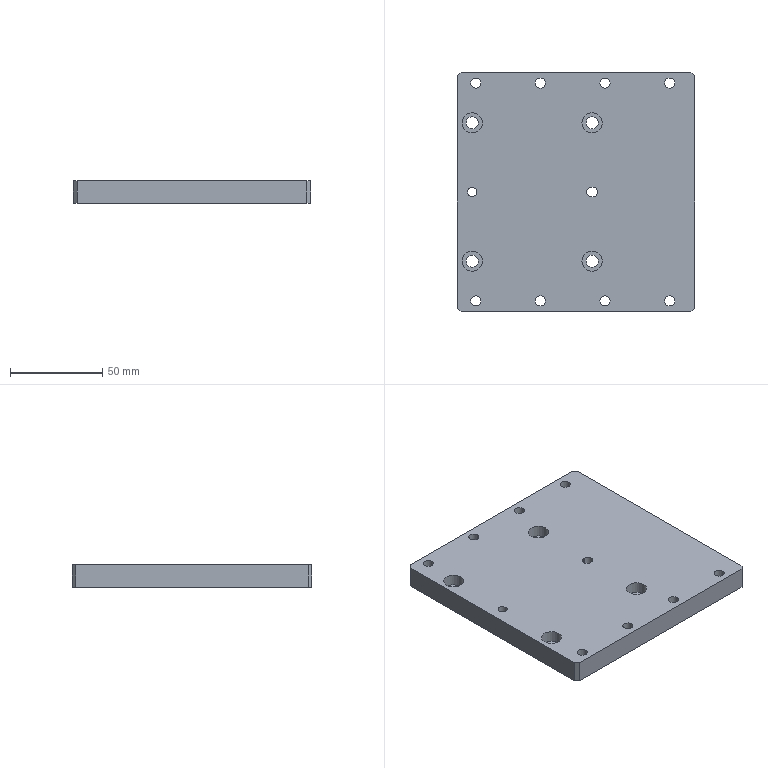CAM job | NX | 3-axis milling, drilling | part box 128.5 x 130 x 12 mm | stock box 133.5 x 135 x 15 mm
Tools:
number,name,description,diameter,corner_radius,flute_length,length,flutes
3,D3,平底铣刀-粗,3.0,0.0,20.0,75.0,2
6,D6,平底铣刀-粗,6.0,0.0,25.0,75.0,2
9,D10,平底铣刀-粗,10.0,0.0,35.0,75.0,2
11,D3-J,平底铣刀-精,3.0,0.0,50.0,75.0,2
7,D6-J,平底铣刀-精,6.0,0.0,25.0,75.0,2
10,D10-J,平底铣刀-精,10.0,0.0,35.0,75.0,2
1,D80R0.8_FACEMILL,圆鼻刀-粗,80.0,0.8,50.0,75.0,2
1,D80R0.8_FACEMILL-J,圆鼻刀-精,80.0,0.8,50.0,75.0,2
2,D6_CHAMFERMILL,倒角刀,6.0,0.0,3.0,25.0,2
23,D5_REAMER,Drilling Tool,5.0,0.0,75.0,100.0,6
17,ZT5.5,钻头,5.5,0.0,35.0,50.0,2
18,ZT6.6,钻头,6.6,0.0,35.0,50.0,2
19,ZT4.9,Drilling Tool,4.9,0.0,35.0,50.0,2
Operations:
program,operation,operation_type,tool,method,geometry_group,spindle_rpm,surface_speed,feed_per_tooth,feed_cut,feed_plunge,cut_length_mm,path_length_mm,cut_time_min,machine_time_min
B,FLOOR-FACE-ROUGHING_COPY,VolumeBased25DMillingOperation,D80R0.8_FACEMILL,LAYERED-ROUGHING-DEPTHK-STEPG,W-B,2800.0,703.696,0.5357,3000.0,100.0,4313.206,5643.292,1.438,1.571
B,FLOOR-FACE-FINISH_COPY,VolumeBased25DMillingOperation,D80R0.8_FACEMILL-J,SIDE-FINISH-DEPTHK-STEPG,W-B,4000.0,1005.28,0.125,1000.0,100.0,718.084,754.084,0.7181,0.7217
B,COUNTERSINK-MILL_1,CylinderMilling,D6,METHOD,W-B,8000.0,150.796,0.125,2000.0,100.0,1699.591,2388.39,0.8498,0.9187
B,HOLE-MILL_1,CylinderMilling,D6-J,METHOD,W-B,8000.0,150.796,0.0375,600.0,100.0,140.453,874.854,0.2341,0.3075
B,DRILL-CHAMFER-DJ10_1,Operation,D6_CHAMFERMILL,METHOD,W-B,8000.0,150.796,0.0625,1000.0,0.0,5.8,51.6,0.0058,0.0104
B,CHAMFER-MILL_4,PlanarMilling,D6_CHAMFERMILL,METHOD,W-B,8000.0,150.796,0.075,1200.0,100.0,81.784,456.231,0.0682,0.1056
B,CHAMFER-MILL_5,PlanarMilling,D6_CHAMFERMILL,METHOD,W-B,8000.0,150.796,0.0375,600.0,100.0,260.714,939.079,0.4345,0.5024
B,C0.3-CLOSED-CONTOUR-CHAMFER-6X45L_COPY,PlanarMilling,D6_CHAMFERMILL,CLIMB_CHAMFER-DEPTH0-STEPG,W-B,7000.0,131.0,0.1071,1500.0,100.0,556.385,724.464,0.3709,0.3877
A,TOP-FACE,FaceMilling,D80R0.8_FACEMILL,SIDE-FINISH-DEPTHK-STEPG,W-A,4000.0,1005.31,0.125,1000.0,100.0,748.25,784.25,0.7482,0.7518
A,OUTLINE-ROUGHING_2,VolumeBased25DMillingOperation,D10,METHOD,W-A,8000.0,251.327,0.3125,5000.0,80.0,9255.594,9306.294,1.851,1.856
A,SPOT-DRILL-DEPTH0.8,Operation,D6_CHAMFERMILL,NONE,W-A,8000.0,150.796,0.0312,500.0,90.0,25.2,550.335,0.0504,0.1029
A,THROUGH-HOLE-5-6,Operation,ZT5.5,NONE,W-A,3000.0,51.836,0.025,150.0,90.0,90.019,555.128,0.6001,0.6466
A,COUNTERSINK-HOLE-DRILL-STAGE0,Operation,ZT6.6,NONE,W-A,1200.0,24.881,0.0625,150.0,90.0,67.931,383.885,0.4529,0.4845
A,THROUGH-HOLE-FINISH-6.0-PRE-DRILL,Operation,ZT4.9,NONE,W-A,2500.0,38.484,0.05,250.0,90.0,34.829,175.166,0.1393,0.1533
A,THROUGH-SLOT-ROUGHING_1,VolumeBased25DMillingOperation,D3,METHOD,W-A,6000.0,56.549,0.0417,500.0,100.0,702.896,753.896,1.406,1.411
A,HOLE-ROUGHING-D6_1,CylinderMilling,D6,NONE,W-A,8000.0,150.796,0.075,1200.0,100.0,923.332,1311.932,0.7694,0.8083
A,HOLE-FINISH-D6_1,CylinderMilling,D6-J,FINISH-STEPDEPTH-OFF,W-A,8000.0,150.796,0.0312,500.0,100.0,178.461,569.061,0.3569,0.396
A,SELECTED-BODY-ONLY,SurfaceContour,D6_CHAMFERMILL,METHOD,W-A,8000.0,150.796,0.1875,3000.0,100.0,548.302,677.285,0.1828,0.1957
A,CHAMFER-MILL_1,PlanarMilling,D6_CHAMFERMILL,METHOD,W-A,8000.0,150.796,0.0312,500.0,100.0,18.482,59.481,0.037,0.0411
A,CHAMFER-MILL_2,PlanarMilling,D6_CHAMFERMILL,METHOD,W-A,8000.0,150.796,0.0312,500.0,100.0,157.506,811.867,0.315,0.3804
A,CHAMFER-MILL_3,PlanarMilling,D6_CHAMFERMILL,NONE,W-A,8000.0,150.796,0.05,800.0,100.0,173.57,518.408,0.217,0.2514
A,SLOT-FINISH_1,VolumeBased25DMillingOperation,D3-J,METHOD,W-A,6000.0,56.549,0.0167,200.0,100.0,31.798,113.599,0.159,0.1672
A,REAM-HOLE,Operation,D5_REAMER,METHOD,W-A,500.0,7.854,0.0167,50.0,0.0,14.0,68.0,0.28,0.2854
A,OUTLINE-SEMI-FINISH_2,VolumeBased25DMillingOperation,D10-J,METHOD,W-A,8000.0,251.327,0.0625,1000.0,100.0,548.688,612.088,0.5487,0.555